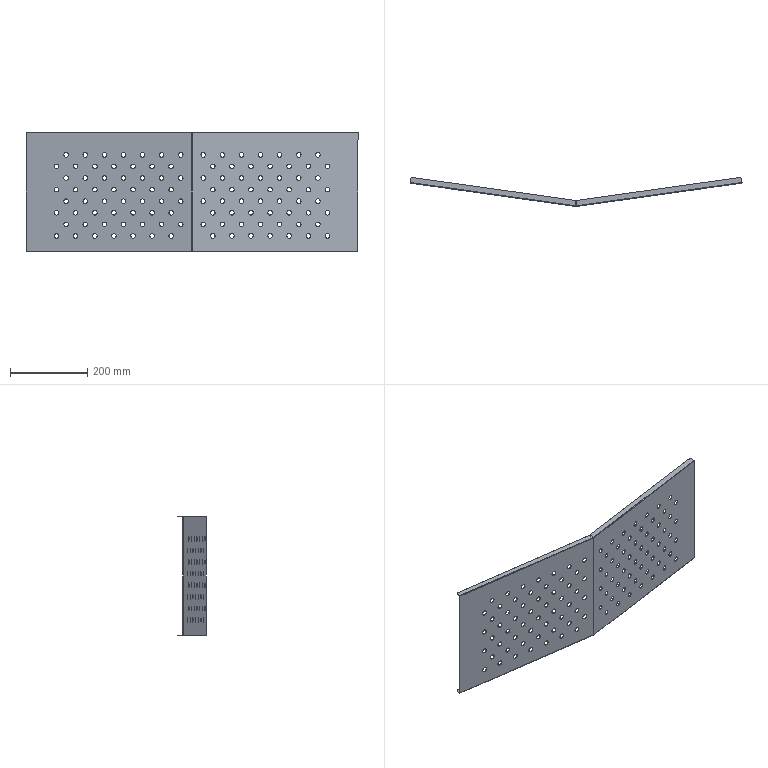Part | SolidWorks | features LPattern 3, ICE 2, EdgeFlange 1, Fillet 1, FlatPattern 1, SMBaseFlange 1, SheetMetal 1 | 1 solid | 276 faces | box 860.334 x 74.65 x 310 mm | volume 335938 mm3 | cylinder 240 | plane 32 | spline 4 | commonest cylinder face diameters 12 x224 10 x6 0.2 x5 2.6 x5